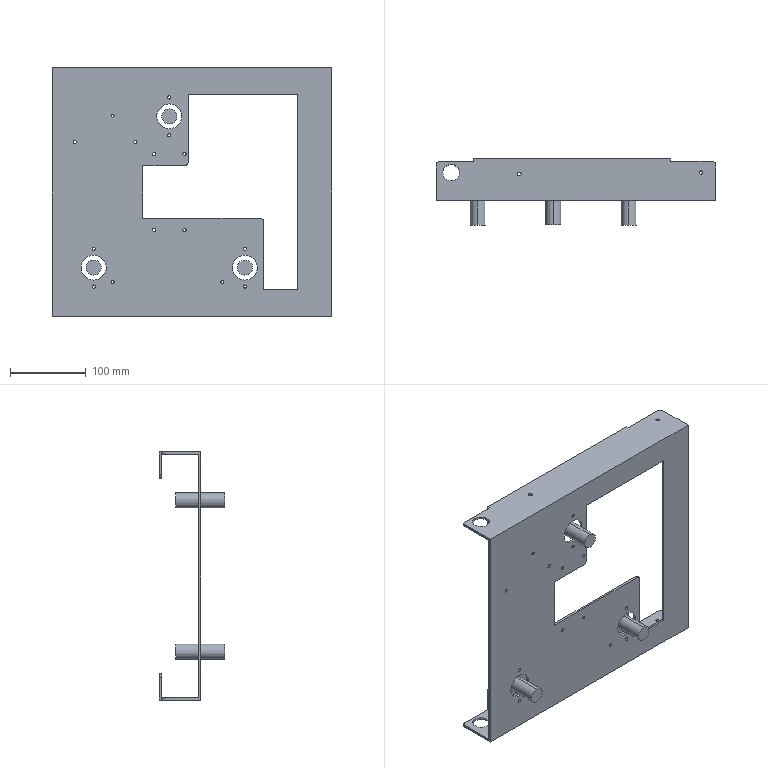Part | SolidWorks | features HoleWzd 7, ICE 7, Cut 2, Fillet 2, Extrusion 1, FlattenBends 1, MirrorPattern 1, MoveFace 1, ProcessBends 1 | 4 solids | 112 faces | box 370 x 87 x 328 mm | volume 480220 mm3 | cylinder 70 | plane 36 | cone 6 | commonest cylinder face diameters 4.2 x24 10 x10 4 x6 5 x6 20 x6 33 x6